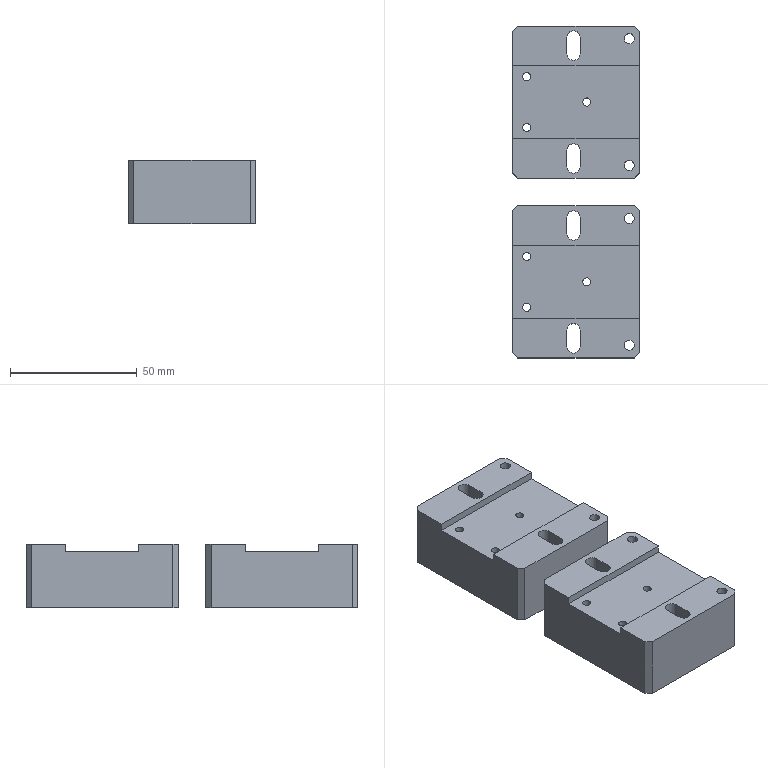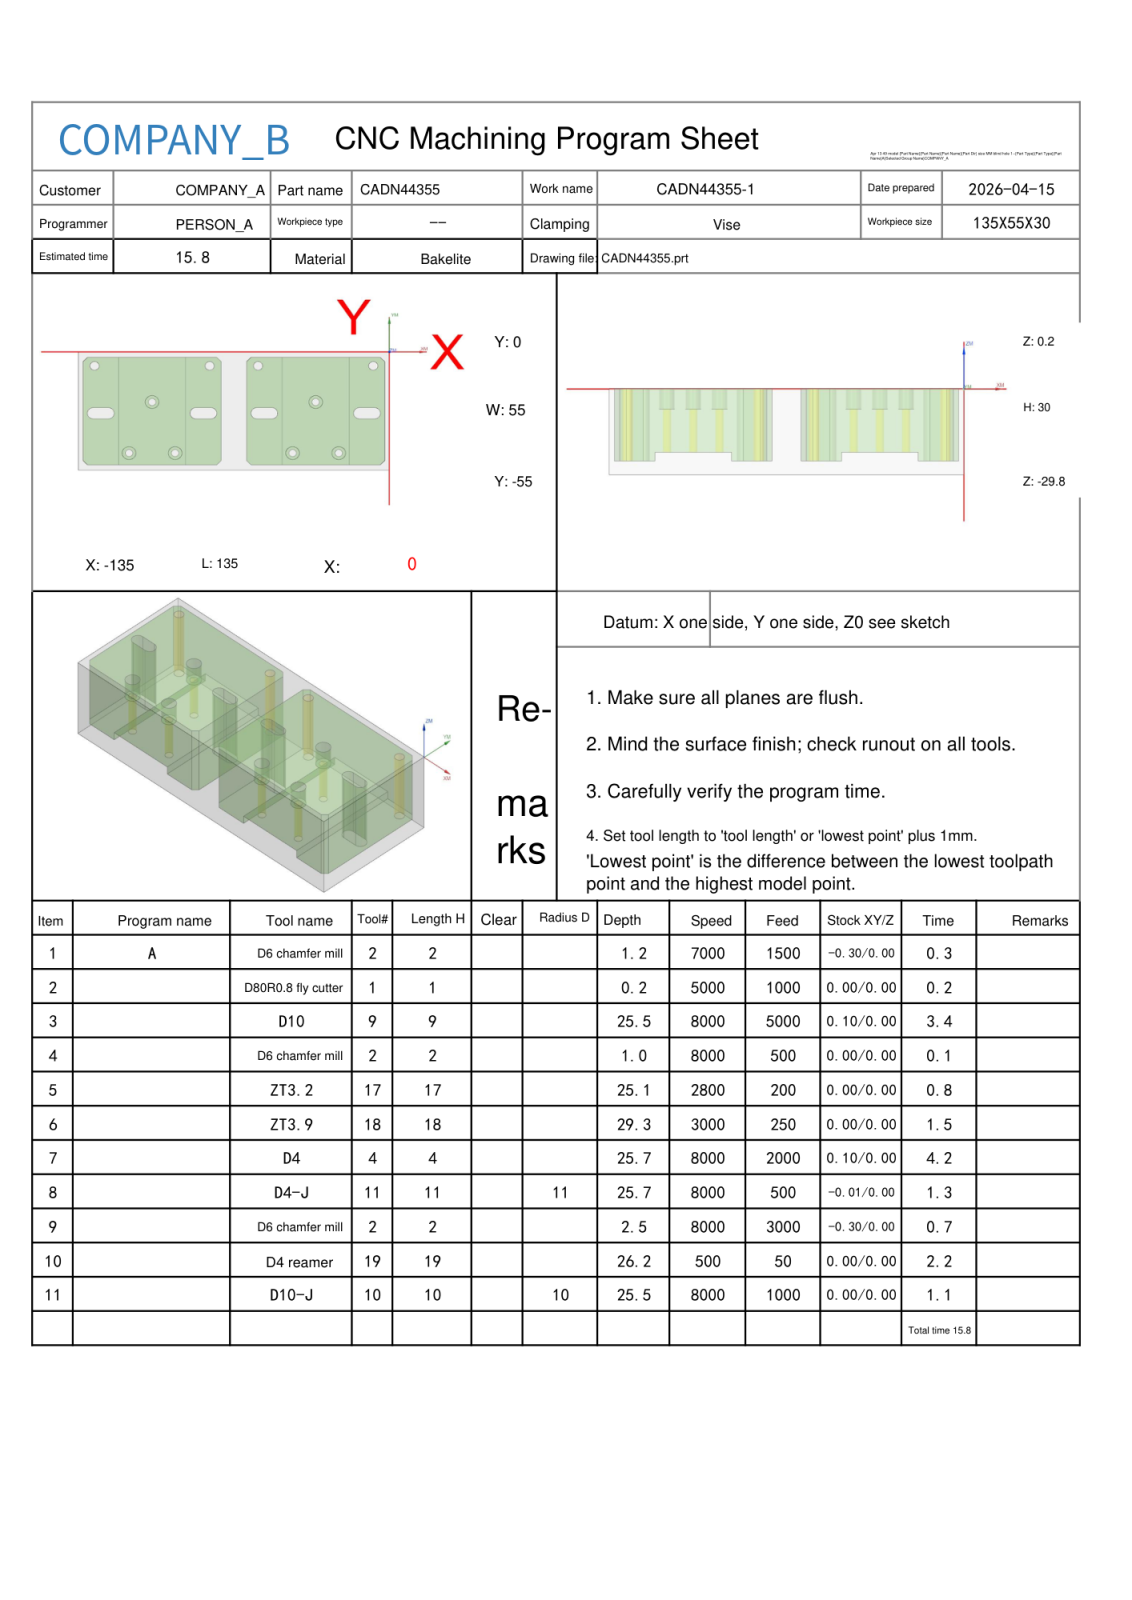NC program | NX | posted by the shop | part box 50 x 131 x 25 mm
Lines 4078 to 5183 of 5183:
N8 T11 M06
(D4-J  D=4. R=0. H=11 ce=0.00 di=0.00)
G00 G90 G54 X-42. Y-47. M03 S8000
G43 H11 Z20.
M08
Z.5
G41 D11
G01 X-41.815 Y-46.923 F500.
G03 X-41.52 Y-46.48 I-.185 J.443
X-42. Y-46. I-.48 J0.0
X-42. Y-46. Z-4.5 I0.0 J-1.
X-42. Y-48. Z-7. I0.0 J-1.
X-41. Y-47. I0.0 J1.
X-42. Y-46. I-1. J0.0
X-43. Y-47. I0.0 J-1.
X-42. Y-48. I1. J0.0
X-41.52 Y-47.52 I0.0 J.48
X-41.815 Y-47.077 I-.48 J0.0
G01 G40 X-42. Y-47.
G00 Z20.
X-22.
Z.5
G41 D11
G01 X-21.815 Y-46.923
G03 X-21.52 Y-46.48 I-.185 J.443
X-22. Y-46. I-.48 J0.0
X-22. Y-46. Z-4.5 I0.0 J-1.
X-22. Y-48. Z-7. I0.0 J-1.
X-21. Y-47. I0.0 J1.
X-22. Y-46. I-1. J0.0
X-23. Y-47. I0.0 J-1.
X-22. Y-48. I1. J0.0
X-21.52 Y-47.52 I0.0 J.48
X-21.815 Y-47.077 I-.48 J0.0
G01 G40 X-22. Y-47.
G00 Z20.
X-32. Y-23.3
Z.5
G41 D11
G01 X-31.815 Y-23.223
G03 X-31.52 Y-22.78 I-.185 J.443
X-32. Y-22.3 I-.48 J0.0
X-32. Y-22.3 Z-4.5 I0.0 J-1.
X-32. Y-24.3 Z-7. I0.0 J-1.
X-31. Y-23.3 I0.0 J1.
X-32. Y-22.3 I-1. J0.0
X-33. Y-23.3 I0.0 J-1.
X-32. Y-24.3 I1. J0.0
X-31.52 Y-23.82 I0.0 J.48
X-31.815 Y-23.377 I-.48 J0.0
G01 G40 X-32. Y-23.3
G00 Z20.
X-93. Y-47.
Z.5
G41 D11
G01 X-92.815 Y-46.923
G03 X-92.52 Y-46.48 I-.185 J.443
X-93. Y-46. I-.48 J0.0
X-93. Y-46. Z-4.5 I0.0 J-1.
X-93. Y-48. Z-7. I0.0 J-1.
X-92. Y-47. I0.0 J1.
X-93. Y-46. I-1. J0.0
X-94. Y-47. I0.0 J-1.
X-93. Y-48. I1. J0.0
X-92.52 Y-47.52 I0.0 J.48
X-92.815 Y-47.077 I-.48 J0.0
G01 G40 X-93. Y-47.
G00 Z20.
X-113.
Z.5
G41 D11
G01 X-112.815 Y-46.923
G03 X-112.52 Y-46.48 I-.185 J.443
X-113. Y-46. I-.48 J0.0
X-113. Y-46. Z-4.5 I0.0 J-1.
X-113. Y-48. Z-7. I0.0 J-1.
X-112. Y-47. I0.0 J1.
X-113. Y-46. I-1. J0.0
X-114. Y-47. I0.0 J-1.
X-113. Y-48. I1. J0.0
X-112.52 Y-47.52 I0.0 J.48
X-112.815 Y-47.077 I-.48 J0.0
G01 G40 X-113. Y-47.
G00 Z20.
X-103. Y-23.3
Z.5
G41 D11
G01 X-102.815 Y-23.223
G03 X-102.52 Y-22.78 I-.185 J.443
X-103. Y-22.3 I-.48 J0.0
X-103. Y-22.3 Z-4.5 I0.0 J-1.
X-103. Y-24.3 Z-7. I0.0 J-1.
X-102. Y-23.3 I0.0 J1.
X-103. Y-22.3 I-1. J0.0
X-104. Y-23.3 I0.0 J-1.
X-103. Y-24.3 I1. J0.0
X-102.52 Y-23.82 I0.0 J.48
X-102.815 Y-23.377 I-.48 J0.0
G01 G40 X-103. Y-23.3
G00 Z20.
G00 G90 X-9.525 Y-28.14 M03 S6000
Z20.
Z-3.75
G01 Z-4.25 F500.
G41 D11
Y-28.09
G03 X-9.725 Y-27.89 I-.2 J0.0
G01 X-12.95
G03 X-13.56 Y-28.5 I0.0 J-.61
X-12.95 Y-29.11 I.61 J0.0
G01 X-6.5
G03 X-5.89 Y-28.5 I0.0 J.61
X-6.5 Y-27.89 I-.61 J0.0
G01 X-9.725
X-10.225
G03 X-10.425 Y-28.09 I0.0 J-.2
G01 G40 Y-28.14
Z-3.75
G00 Z1.
X-9.525
Z-8.
G01 Z-8.5
G41 D11
Y-28.09
G03 X-9.725 Y-27.89 I-.2 J0.0
G01 X-12.95
G03 X-13.56 Y-28.5 I0.0 J-.61
X-12.95 Y-29.11 I.61 J0.0
G01 X-6.5
G03 X-5.89 Y-28.5 I0.0 J.61
X-6.5 Y-27.89 I-.61 J0.0
G01 X-9.725
X-10.225
G03 X-10.425 Y-28.09 I0.0 J-.2
G01 G40 Y-28.14
Z-8.
G00 Z-3.25
X-9.525
Z-12.25
G01 Z-12.75
G41 D11
Y-28.09
G03 X-9.725 Y-27.89 I-.2 J0.0
G01 X-12.95
G03 X-13.56 Y-28.5 I0.0 J-.61
X-12.95 Y-29.11 I.61 J0.0
G01 X-6.5
G03 X-5.89 Y-28.5 I0.0 J.61
X-6.5 Y-27.89 I-.61 J0.0
G01 X-9.725
X-10.225
G03 X-10.425 Y-28.09 I0.0 J-.2
G01 G40 Y-28.14
Z-12.25
G00 Z-7.5
X-9.525
Z-16.5
G01 Z-17.
G41 D11
Y-28.09
G03 X-9.725 Y-27.89 I-.2 J0.0
G01 X-12.95
G03 X-13.56 Y-28.5 I0.0 J-.61
X-12.95 Y-29.11 I.61 J0.0
G01 X-6.5
G03 X-5.89 Y-28.5 I0.0 J.61
X-6.5 Y-27.89 I-.61 J0.0
G01 X-9.725
X-10.225
G03 X-10.425 Y-28.09 I0.0 J-.2
G01 G40 Y-28.14
Z-16.5
G00 Z-11.75
X-9.525
Z-20.75
G01 Z-21.25
G41 D11
Y-28.09
G03 X-9.725 Y-27.89 I-.2 J0.0
G01 X-12.95
G03 X-13.56 Y-28.5 I0.0 J-.61
X-12.95 Y-29.11 I.61 J0.0
G01 X-6.5
G03 X-5.89 Y-28.5 I0.0 J.61
X-6.5 Y-27.89 I-.61 J0.0
G01 X-9.725
X-10.225
G03 X-10.425 Y-28.09 I0.0 J-.2
G01 G40 Y-28.14
Z-20.75
G00 Z-16.
X-9.525
Z-25.
G01 Z-25.5
G41 D11
Y-28.09
G03 X-9.725 Y-27.89 I-.2 J0.0
G01 X-12.95
G03 X-13.56 Y-28.5 I0.0 J-.61
X-12.95 Y-29.11 I.61 J0.0
G01 X-6.5
G03 X-5.89 Y-28.5 I0.0 J.61
X-6.5 Y-27.89 I-.61 J0.0
G01 X-9.725
X-10.225
G03 X-10.425 Y-28.09 I0.0 J-.2
G01 G40 Y-28.14
Z-25.
G00 Z20.
X-54.475 Y-28.86
Z-3.75
G01 Z-4.25
G41 D11
Y-28.91
G03 X-54.275 Y-29.11 I.2 J0.0
G01 X-51.05
G03 X-50.44 Y-28.5 I0.0 J.61
X-51.05 Y-27.89 I-.61 J0.0
G01 X-57.5
G03 X-58.11 Y-28.5 I0.0 J-.61
X-57.5 Y-29.11 I.61 J0.0
G01 X-54.275
X-53.775
G03 X-53.575 Y-28.91 I0.0 J.2
G01 G40 Y-28.86
Z-3.75
G00 Z1.
X-54.475
Z-8.
G01 Z-8.5
G41 D11
Y-28.91
G03 X-54.275 Y-29.11 I.2 J0.0
G01 X-51.05
G03 X-50.44 Y-28.5 I0.0 J.61
X-51.05 Y-27.89 I-.61 J0.0
G01 X-57.5
G03 X-58.11 Y-28.5 I0.0 J-.61
X-57.5 Y-29.11 I.61 J0.0
G01 X-54.275
X-53.775
G03 X-53.575 Y-28.91 I0.0 J.2
G01 G40 Y-28.86
Z-8.
G00 Z-3.25
X-54.475
Z-12.25
G01 Z-12.75
G41 D11
Y-28.91
G03 X-54.275 Y-29.11 I.2 J0.0
G01 X-51.05
G03 X-50.44 Y-28.5 I0.0 J.61
X-51.05 Y-27.89 I-.61 J0.0
G01 X-57.5
G03 X-58.11 Y-28.5 I0.0 J-.61
X-57.5 Y-29.11 I.61 J0.0
G01 X-54.275
X-53.775
G03 X-53.575 Y-28.91 I0.0 J.2
G01 G40 Y-28.86
Z-12.25
G00 Z-7.5
X-54.475
Z-16.5
G01 Z-17.
G41 D11
Y-28.91
G03 X-54.275 Y-29.11 I.2 J0.0
G01 X-51.05
G03 X-50.44 Y-28.5 I0.0 J.61
X-51.05 Y-27.89 I-.61 J0.0
G01 X-57.5
G03 X-58.11 Y-28.5 I0.0 J-.61
X-57.5 Y-29.11 I.61 J0.0
G01 X-54.275
X-53.775
G03 X-53.575 Y-28.91 I0.0 J.2
G01 G40 Y-28.86
Z-16.5
G00 Z-11.75
X-54.475
Z-20.75
G01 Z-21.25
G41 D11
Y-28.91
G03 X-54.275 Y-29.11 I.2 J0.0
G01 X-51.05
G03 X-50.44 Y-28.5 I0.0 J.61
X-51.05 Y-27.89 I-.61 J0.0
G01 X-57.5
G03 X-58.11 Y-28.5 I0.0 J-.61
X-57.5 Y-29.11 I.61 J0.0
G01 X-54.275
X-53.775
G03 X-53.575 Y-28.91 I0.0 J.2
G01 G40 Y-28.86
Z-20.75
G00 Z-16.
X-54.475
Z-25.
G01 Z-25.5
G41 D11
Y-28.91
G03 X-54.275 Y-29.11 I.2 J0.0
G01 X-51.05
G03 X-50.44 Y-28.5 I0.0 J.61
X-51.05 Y-27.89 I-.61 J0.0
G01 X-57.5
G03 X-58.11 Y-28.5 I0.0 J-.61
X-57.5 Y-29.11 I.61 J0.0
G01 X-54.275
X-53.775
G03 X-53.575 Y-28.91 I0.0 J.2
G01 G40 Y-28.86
Z-25.
G00 Z20.
X-80.925
Z-3.75
G01 Z-4.25
G41 D11
Y-28.91
G03 X-80.725 Y-29.11 I.2 J0.0
G01 X-77.5
G03 X-76.89 Y-28.5 I0.0 J.61
X-77.5 Y-27.89 I-.61 J0.0
G01 X-83.95
G03 X-84.56 Y-28.5 I0.0 J-.61
X-83.95 Y-29.11 I.61 J0.0
G01 X-80.725
X-80.225
G03 X-80.025 Y-28.91 I0.0 J.2
G01 G40 Y-28.86
Z-3.75
G00 Z1.
X-80.925
Z-8.
G01 Z-8.5
G41 D11
Y-28.91
G03 X-80.725 Y-29.11 I.2 J0.0
G01 X-77.5
G03 X-76.89 Y-28.5 I0.0 J.61
X-77.5 Y-27.89 I-.61 J0.0
G01 X-83.95
G03 X-84.56 Y-28.5 I0.0 J-.61
X-83.95 Y-29.11 I.61 J0.0
G01 X-80.725
X-80.225
G03 X-80.025 Y-28.91 I0.0 J.2
G01 G40 Y-28.86
Z-8.
G00 Z-3.25
X-80.925
Z-12.25
G01 Z-12.75
G41 D11
Y-28.91
G03 X-80.725 Y-29.11 I.2 J0.0
G01 X-77.5
G03 X-76.89 Y-28.5 I0.0 J.61
X-77.5 Y-27.89 I-.61 J0.0
G01 X-83.95
G03 X-84.56 Y-28.5 I0.0 J-.61
X-83.95 Y-29.11 I.61 J0.0
G01 X-80.725
X-80.225
G03 X-80.025 Y-28.91 I0.0 J.2
G01 G40 Y-28.86
Z-12.25
G00 Z-7.5
X-80.925
Z-16.5
G01 Z-17.
G41 D11
Y-28.91
G03 X-80.725 Y-29.11 I.2 J0.0
G01 X-77.5
G03 X-76.89 Y-28.5 I0.0 J.61
X-77.5 Y-27.89 I-.61 J0.0
G01 X-83.95
G03 X-84.56 Y-28.5 I0.0 J-.61
X-83.95 Y-29.11 I.61 J0.0
G01 X-80.725
X-80.225
G03 X-80.025 Y-28.91 I0.0 J.2
G01 G40 Y-28.86
Z-16.5
G00 Z-11.75
X-80.925
Z-20.75
G01 Z-21.25
G41 D11
Y-28.91
G03 X-80.725 Y-29.11 I.2 J0.0
G01 X-77.5
G03 X-76.89 Y-28.5 I0.0 J.61
X-77.5 Y-27.89 I-.61 J0.0
G01 X-83.95
G03 X-84.56 Y-28.5 I0.0 J-.61
X-83.95 Y-29.11 I.61 J0.0
G01 X-80.725
X-80.225
G03 X-80.025 Y-28.91 I0.0 J.2
G01 G40 Y-28.86
Z-20.75
G00 Z-16.
X-80.925
Z-25.
G01 Z-25.5
G41 D11
Y-28.91
G03 X-80.725 Y-29.11 I.2 J0.0
G01 X-77.5
G03 X-76.89 Y-28.5 I0.0 J.61
X-77.5 Y-27.89 I-.61 J0.0
G01 X-83.95
G03 X-84.56 Y-28.5 I0.0 J-.61
X-83.95 Y-29.11 I.61 J0.0
G01 X-80.725
X-80.225
G03 X-80.025 Y-28.91 I0.0 J.2
G01 G40 Y-28.86
Z-25.
G00 Z20.
X-125.075 Y-28.14
Z-3.75
G01 Z-4.25
G41 D11
Y-28.09
G03 X-125.275 Y-27.89 I-.2 J0.0
G01 X-128.5
G03 X-129.11 Y-28.5 I0.0 J-.61
X-128.5 Y-29.11 I.61 J0.0
G01 X-122.05
G03 X-121.44 Y-28.5 I0.0 J.61
X-122.05 Y-27.89 I-.61 J0.0
G01 X-125.275
X-125.775
G03 X-125.975 Y-28.09 I0.0 J-.2
G01 G40 Y-28.14
Z-3.75
G00 Z1.
X-125.075
Z-8.
G01 Z-8.5
G41 D11
Y-28.09
G03 X-125.275 Y-27.89 I-.2 J0.0
G01 X-128.5
G03 X-129.11 Y-28.5 I0.0 J-.61
X-128.5 Y-29.11 I.61 J0.0
G01 X-122.05
G03 X-121.44 Y-28.5 I0.0 J.61
X-122.05 Y-27.89 I-.61 J0.0
G01 X-125.275
X-125.775
G03 X-125.975 Y-28.09 I0.0 J-.2
G01 G40 Y-28.14
Z-8.
G00 Z-3.25
X-125.075
Z-12.25
G01 Z-12.75
G41 D11
Y-28.09
G03 X-125.275 Y-27.89 I-.2 J0.0
G01 X-128.5
G03 X-129.11 Y-28.5 I0.0 J-.61
X-128.5 Y-29.11 I.61 J0.0
G01 X-122.05
G03 X-121.44 Y-28.5 I0.0 J.61
X-122.05 Y-27.89 I-.61 J0.0
G01 X-125.275
X-125.775
G03 X-125.975 Y-28.09 I0.0 J-.2
G01 G40 Y-28.14
Z-12.25
G00 Z-7.5
X-125.075
Z-16.5
G01 Z-17.
G41 D11
Y-28.09
G03 X-125.275 Y-27.89 I-.2 J0.0
G01 X-128.5
G03 X-129.11 Y-28.5 I0.0 J-.61
X-128.5 Y-29.11 I.61 J0.0
G01 X-122.05
G03 X-121.44 Y-28.5 I0.0 J.61
X-122.05 Y-27.89 I-.61 J0.0
G01 X-125.275
X-125.775
G03 X-125.975 Y-28.09 I0.0 J-.2
G01 G40 Y-28.14
Z-16.5
G00 Z-11.75
X-125.075
Z-20.75
G01 Z-21.25
G41 D11
Y-28.09
G03 X-125.275 Y-27.89 I-.2 J0.0
G01 X-128.5
G03 X-129.11 Y-28.5 I0.0 J-.61
X-128.5 Y-29.11 I.61 J0.0
G01 X-122.05
G03 X-121.44 Y-28.5 I0.0 J.61
X-122.05 Y-27.89 I-.61 J0.0
G01 X-125.275
X-125.775
G03 X-125.975 Y-28.09 I0.0 J-.2
G01 G40 Y-28.14
Z-20.75
G00 Z-16.
X-125.075
Z-25.
G01 Z-25.5
G41 D11
Y-28.09
G03 X-125.275 Y-27.89 I-.2 J0.0
G01 X-128.5
G03 X-129.11 Y-28.5 I0.0 J-.61
X-128.5 Y-29.11 I.61 J0.0
G01 X-122.05
G03 X-121.44 Y-28.5 I0.0 J.61
X-122.05 Y-27.89 I-.61 J0.0
G01 X-125.275
X-125.775
G03 X-125.975 Y-28.09 I0.0 J-.2
G01 G40 Y-28.14
Z-25.
G00 Z20.
G91 G28 Z0.0
M05
M09
G91 G28 Z0.0
M01
N9 T02 M06
(D6 chamfer mill  D=6. R=0. H=02 ce=0.00 di=0.00)
G00 G90 G54 X-31.75 Y-54.628 M03 S8000
G43 H02 Z20.
M08
Z2.099
G01 Z-1.5 F3000.
G03 X-31.67 Y-54.328 I-.52 J.3
X-31.97 Y-53.808 I-.6 J0.0
G01 X-32. Y-53.8
X-60.
X-60.254 Y-53.775
X-60.497 Y-53.701
X-60.722 Y-53.581
X-60.919 Y-53.419
X-62.919 Y-51.419
X-63.081 Y-51.222
X-63.201 Y-50.997
X-63.275 Y-50.754
X-63.3 Y-50.5
Y-4.5
X-63.275 Y-4.246
X-63.201 Y-4.003
X-63.081 Y-3.778
X-62.919 Y-3.581
X-60.919 Y-1.581
X-60.722 Y-1.419
X-60.497 Y-1.299
X-60.254 Y-1.225
X-60. Y-1.2
X-4.
X-3.746 Y-1.225
X-3.503 Y-1.299
X-3.278 Y-1.419
X-3.081 Y-1.581
X-1.081 Y-3.581
X-.919 Y-3.778
X-.799 Y-4.003
X-.725 Y-4.246
X-.7 Y-4.5
Y-50.5
X-.725 Y-50.754
X-.799 Y-50.997
X-.919 Y-51.222
X-1.081 Y-51.419
X-3.081 Y-53.419
X-3.278 Y-53.581
X-3.503 Y-53.701
X-3.746 Y-53.775
X-4. Y-53.8
X-32.
X-32.03 Y-53.808
G03 X-32.33 Y-54.328 I.3 J-.52
X-32.25 Y-54.628 I.6 J0.0
G01 Z2.099
G00 Z20.
X-9.475 Y-28.028
Z2.099
G01 Z-1.5
G03 X-9.395 Y-27.728 I-.52 J.3
X-9.695 Y-27.208 I-.6 J0.0
G01 X-9.725 Y-27.2
X-12.95
G03 X-14.25 Y-28.5 I0.0 J-1.3
X-12.95 Y-29.8 I1.3 J0.0
G01 X-6.5
G03 X-5.2 Y-28.5 I0.0 J1.3
X-6.5 Y-27.2 I-1.3 J0.0
G01 X-9.725
X-9.755 Y-27.208
G03 X-10.055 Y-27.728 I.3 J-.52
X-9.975 Y-28.028 I.6 J0.0
G01 Z2.099
G00 Z20.
X-54.025
Z2.099
G01 Z-1.5
G03 X-53.945 Y-27.728 I-.52 J.3
X-54.245 Y-27.208 I-.6 J0.0
G01 X-54.275 Y-27.2
X-57.5
G03 X-58.8 Y-28.5 I0.0 J-1.3
X-57.5 Y-29.8 I1.3 J0.0
G01 X-51.05
G03 X-49.75 Y-28.5 I0.0 J1.3
X-51.05 Y-27.2 I-1.3 J0.0
G01 X-54.275
X-54.305 Y-27.208
G03 X-54.605 Y-27.728 I.3 J-.52
X-54.525 Y-28.028 I.6 J0.0
G01 Z2.099
G00 Z20.
X-102.75 Y-54.628
Z2.099
G01 Z-1.5
G03 X-102.67 Y-54.328 I-.52 J.3
X-102.97 Y-53.808 I-.6 J0.0
G01 X-103. Y-53.8
X-131.
X-131.254 Y-53.775
X-131.497 Y-53.701
X-131.722 Y-53.581
X-131.919 Y-53.419
X-133.919 Y-51.419
X-134.081 Y-51.222
X-134.201 Y-50.997
X-134.275 Y-50.754
X-134.3 Y-50.5
Y-4.5
X-134.275 Y-4.246
X-134.201 Y-4.003
X-134.081 Y-3.778
X-133.919 Y-3.581
X-131.919 Y-1.581
X-131.722 Y-1.419
X-131.497 Y-1.299
X-131.254 Y-1.225
X-131. Y-1.2
X-75.
X-74.746 Y-1.225
X-74.503 Y-1.299
X-74.278 Y-1.419
X-74.081 Y-1.581
X-72.081 Y-3.581
X-71.919 Y-3.778
X-71.799 Y-4.003
X-71.725 Y-4.246
X-71.7 Y-4.5
Y-50.5
X-71.725 Y-50.754
X-71.799 Y-50.997
X-71.919 Y-51.222
X-72.081 Y-51.419
X-74.081 Y-53.419
X-74.278 Y-53.581
X-74.503 Y-53.701
X-74.746 Y-53.775
X-75. Y-53.8
X-103.
X-103.03 Y-53.808
G03 X-103.33 Y-54.328 I.3 J-.52
X-103.25 Y-54.628 I.6 J0.0
G01 Z2.099
G00 Z20.
X-80.475 Y-28.028
Z2.099
G01 Z-1.5
G03 X-80.395 Y-27.728 I-.52 J.3
X-80.695 Y-27.208 I-.6 J0.0
G01 X-80.725 Y-27.2
X-83.95
G03 X-85.25 Y-28.5 I0.0 J-1.3
X-83.95 Y-29.8 I1.3 J0.0
G01 X-77.5
G03 X-76.2 Y-28.5 I0.0 J1.3
X-77.5 Y-27.2 I-1.3 J0.0
G01 X-80.725
X-80.755 Y-27.208
G03 X-81.055 Y-27.728 I.3 J-.52
X-80.975 Y-28.028 I.6 J0.0
G01 Z2.099
G00 Z20.
X-125.025
Z2.099
G01 Z-1.5
G03 X-124.945 Y-27.728 I-.52 J.3
X-125.245 Y-27.208 I-.6 J0.0
G01 X-125.275 Y-27.2
X-128.5
G03 X-129.8 Y-28.5 I0.0 J-1.3
X-128.5 Y-29.8 I1.3 J0.0
G01 X-122.05
G03 X-120.75 Y-28.5 I0.0 J1.3
X-122.05 Y-27.2 I-1.3 J0.0
G01 X-125.275
X-125.305 Y-27.208
G03 X-125.605 Y-27.728 I.3 J-.52
X-125.525 Y-28.028 I.6 J0.0
G01 Z2.099
G00 Z20.
G00 G90 X-7. Y-6.5 M03 S8000
Z20.
G98 G81 X-7. Y-6.5 Z-2.3 R3. F500.
X-57.
X-78.
X-128.
G80
G00 Z20.
G00 G90 X-101.019 Y-22.13 M03 S8000
Z20.
Z2.5
G01 X-101.067 Y-22.048 Z2.465 F500.
X-101.264 Y-21.787 Z2.346
X-101.496 Y-21.556 Z2.227
X-101.759 Y-21.36 Z2.108
X-102.046 Y-21.204 Z1.989
X-102.353 Y-21.09 Z1.87
X-102.673 Y-21.02 Z1.75
X-103. Y-20.997 Z1.631
X-103.327 Y-21.02 Z1.512
X-103.647 Y-21.09 Z1.393
X-103.954 Y-21.204 Z1.274
X-104.241 Y-21.36 Z1.154
X-104.504 Y-21.556 Z1.035
X-104.736 Y-21.787 Z.916
X-104.933 Y-22.048 Z.797
X-105.051 Y-22.252 Z.711
X-105.179 Y-22.553 Z.592
X-105.262 Y-22.87 Z.473
X-105.301 Y-23.195 Z.354
X-105.292 Y-23.522 Z.235
X-105.238 Y-23.845 Z.115
X-105.138 Y-24.157 Z-.004
X-104.994 Y-24.452 Z-.123
X-104.811 Y-24.723 Z-.242
X-104.591 Y-24.965 Z-.361
X-104.339 Y-25.174 Z-.48
X-104.059 Y-25.345 Z-.6
X-103.759 Y-25.474 Z-.719
X-103.443 Y-25.56 Z-.838
X-103.118 Y-25.6 Z-.957
X-103. Z-1.
G03 X-100.7 Y-23.3 I0.0 J2.3
X-103. Y-21. I-2.3 J0.0
X-105.3 Y-23.3 I0.0 J-2.3
X-103. Y-25.6 I2.3 J0.0
X-102.504 Y-25.546 I0.0 J2.3
G01 Z1.5
G00 Z20.
X-111.019 Y-45.83
Z2.5
G01 X-111.067 Y-45.748 Z2.465
X-111.264 Y-45.487 Z2.346
X-111.496 Y-45.256 Z2.227
X-111.759 Y-45.06 Z2.108
X-112.046 Y-44.904 Z1.989
X-112.353 Y-44.79 Z1.87
X-112.673 Y-44.72 Z1.75
X-113. Y-44.697 Z1.631
X-113.327 Y-44.72 Z1.512
X-113.647 Y-44.79 Z1.393
X-113.954 Y-44.904 Z1.274
X-114.241 Y-45.06 Z1.154
X-114.504 Y-45.256 Z1.035
X-114.736 Y-45.487 Z.916
X-114.933 Y-45.748 Z.797
X-115.051 Y-45.952 Z.711
X-115.179 Y-46.253 Z.592
X-115.262 Y-46.57 Z.473
X-115.301 Y-46.895 Z.354
X-115.292 Y-47.222 Z.235
X-115.238 Y-47.545 Z.115
X-115.138 Y-47.857 Z-.004
X-114.994 Y-48.152 Z-.123
X-114.811 Y-48.423 Z-.242
X-114.591 Y-48.665 Z-.361
X-114.339 Y-48.874 Z-.48
X-114.059 Y-49.045 Z-.6
X-113.759 Y-49.174 Z-.719
X-113.443 Y-49.26 Z-.838
X-113.118 Y-49.3 Z-.957
X-113. Z-1.
G03 X-110.7 Y-47. I0.0 J2.3
X-113. Y-44.7 I-2.3 J0.0
X-115.3 Y-47. I0.0 J-2.3
X-113. Y-49.3 I2.3 J0.0
X-112.504 Y-49.246 I0.0 J2.3
G01 Z1.5
G00 Z20.
X-91.019 Y-45.83
Z2.5
G01 X-91.067 Y-45.748 Z2.465
X-91.264 Y-45.487 Z2.346
X-91.496 Y-45.256 Z2.227
X-91.759 Y-45.06 Z2.108
X-92.046 Y-44.904 Z1.989
X-92.353 Y-44.79 Z1.87
X-92.673 Y-44.72 Z1.75
X-93. Y-44.697 Z1.631
X-93.327 Y-44.72 Z1.512
X-93.647 Y-44.79 Z1.393
X-93.954 Y-44.904 Z1.274
X-94.241 Y-45.06 Z1.154
X-94.504 Y-45.256 Z1.035
X-94.736 Y-45.487 Z.916
X-94.933 Y-45.748 Z.797
X-95.051 Y-45.952 Z.711
X-95.179 Y-46.253 Z.592
X-95.262 Y-46.57 Z.473
X-95.301 Y-46.895 Z.354
X-95.292 Y-47.222 Z.235
X-95.238 Y-47.545 Z.115
X-95.138 Y-47.857 Z-.004
X-94.994 Y-48.152 Z-.123
X-94.811 Y-48.423 Z-.242
X-94.591 Y-48.665 Z-.361
X-94.339 Y-48.874 Z-.48
X-94.059 Y-49.045 Z-.6
X-93.759 Y-49.174 Z-.719
X-93.443 Y-49.26 Z-.838
X-93.118 Y-49.3 Z-.957
X-93. Z-1.
G03 X-90.7 Y-47. I0.0 J2.3
X-93. Y-44.7 I-2.3 J0.0
X-95.3 Y-47. I0.0 J-2.3
X-93. Y-49.3 I2.3 J0.0
X-92.504 Y-49.246 I0.0 J2.3
G01 Z1.5
G00 Z20.
X-40.019 Y-45.83
Z2.5
G01 X-40.067 Y-45.748 Z2.465
X-40.264 Y-45.487 Z2.346
X-40.496 Y-45.256 Z2.227
X-40.759 Y-45.06 Z2.108
X-41.046 Y-44.904 Z1.989
X-41.353 Y-44.79 Z1.87
X-41.673 Y-44.72 Z1.75
X-42. Y-44.697 Z1.631
X-42.327 Y-44.72 Z1.512
X-42.647 Y-44.79 Z1.393
X-42.954 Y-44.904 Z1.274
X-43.241 Y-45.06 Z1.154
X-43.504 Y-45.256 Z1.035
X-43.736 Y-45.487 Z.916
X-43.933 Y-45.748 Z.797
X-44.051 Y-45.952 Z.711
X-44.179 Y-46.253 Z.592
X-44.262 Y-46.57 Z.473
X-44.301 Y-46.895 Z.354
X-44.292 Y-47.222 Z.235
X-44.238 Y-47.545 Z.115
X-44.138 Y-47.857 Z-.004
X-43.994 Y-48.152 Z-.123
X-43.811 Y-48.423 Z-.242
X-43.591 Y-48.665 Z-.361
X-43.339 Y-48.874 Z-.48
X-43.059 Y-49.045 Z-.6
X-42.759 Y-49.174 Z-.719
X-42.443 Y-49.26 Z-.838
X-42.118 Y-49.3 Z-.957
X-42. Z-1.
G03 X-39.7 Y-47. I0.0 J2.3
X-42. Y-44.7 I-2.3 J0.0
X-44.3 Y-47. I0.0 J-2.3
X-42. Y-49.3 I2.3 J0.0
X-41.504 Y-49.246 I0.0 J2.3
G01 Z1.5
G00 Z20.
X-20.019 Y-45.83
Z2.5
G01 X-20.067 Y-45.748 Z2.465
X-20.264 Y-45.487 Z2.346
X-20.496 Y-45.256 Z2.227
X-20.759 Y-45.06 Z2.108
X-21.046 Y-44.904 Z1.989
X-21.353 Y-44.79 Z1.87
X-21.673 Y-44.72 Z1.75
X-22. Y-44.697 Z1.631
X-22.327 Y-44.72 Z1.512
X-22.647 Y-44.79 Z1.393
X-22.954 Y-44.904 Z1.274
X-23.241 Y-45.06 Z1.154
X-23.504 Y-45.256 Z1.035
X-23.736 Y-45.487 Z.916
X-23.933 Y-45.748 Z.797
X-24.051 Y-45.952 Z.711
X-24.179 Y-46.253 Z.592
X-24.262 Y-46.57 Z.473
X-24.301 Y-46.895 Z.354
X-24.292 Y-47.222 Z.235
X-24.238 Y-47.545 Z.115
X-24.138 Y-47.857 Z-.004
X-23.994 Y-48.152 Z-.123
X-23.811 Y-48.423 Z-.242
X-23.591 Y-48.665 Z-.361
X-23.339 Y-48.874 Z-.48
X-23.059 Y-49.045 Z-.6
X-22.759 Y-49.174 Z-.719
X-22.443 Y-49.26 Z-.838
X-22.118 Y-49.3 Z-.957
X-22. Z-1.
G03 X-19.7 Y-47. I0.0 J2.3
X-22. Y-44.7 I-2.3 J0.0
X-24.3 Y-47. I0.0 J-2.3
X-22. Y-49.3 I2.3 J0.0
X-21.504 Y-49.246 I0.0 J2.3
G01 Z1.5
G00 Z20.
X-30.019 Y-22.13
Z2.5
G01 X-30.067 Y-22.048 Z2.465
X-30.264 Y-21.787 Z2.346
X-30.496 Y-21.556 Z2.227
X-30.759 Y-21.36 Z2.108
X-31.046 Y-21.204 Z1.989
X-31.353 Y-21.09 Z1.87
X-31.673 Y-21.02 Z1.75
X-32. Y-20.997 Z1.631
X-32.327 Y-21.02 Z1.512
X-32.647 Y-21.09 Z1.393
X-32.954 Y-21.204 Z1.274
X-33.241 Y-21.36 Z1.154
X-33.504 Y-21.556 Z1.035
X-33.736 Y-21.787 Z.916
X-33.933 Y-22.048 Z.797
X-34.051 Y-22.252 Z.711
X-34.179 Y-22.553 Z.592
X-34.262 Y-22.87 Z.473
X-34.301 Y-23.195 Z.354
X-34.292 Y-23.522 Z.235
X-34.238 Y-23.845 Z.115
X-34.138 Y-24.157 Z-.004
X-33.994 Y-24.452 Z-.123
X-33.811 Y-24.723 Z-.242
X-33.591 Y-24.965 Z-.361
X-33.339 Y-25.174 Z-.48
X-33.059 Y-25.345 Z-.6
X-32.759 Y-25.474 Z-.719
X-32.443 Y-25.56 Z-.838
X-32.118 Y-25.6 Z-.957
X-32. Z-1.
G03 X-29.7 Y-23.3 I0.0 J2.3
X-32. Y-21. I-2.3 J0.0
X-34.3 Y-23.3 I0.0 J-2.3
X-32. Y-25.6 I2.3 J0.0
X-31.504 Y-25.546 I0.0 J2.3
G01 Z1.5
G00 Z20.
G91 G28 Z0.0
M05
M09
G91 G28 Z0.0
M01
N10 T19 M06
(D4 reamer D=4. DR_a=180 H=19)
G00 G90 G54 X-7. Y-6.5 M03 S500
G43 H19 Z20.
M08
G98 G81 X-7. Y-6.5 Z-26. R1. F50.
X-57.
X-78.
X-128.
G80
G00 Z20.
G91 G28 Z0.0
M05
M09
G91 G28 Z0.0
M01
N11 T10 M06
(D10-J  D=10. R=0. H=10 ce=0.00 di=0.00)
G00 G90 G54 X-61.013 Y3.616 M03 S8000
G43 H10 Z20.
M08
Z-12.15
G01 Z-12.65 F1000.
G41 D10
X-60.997 Y3.417
G03 X-60. Y2.5 I.997 J.083
G01 X-4.
G02 X-.464 Y1.036 I0.0 J-5.
G01 X1.536 Y-.964
G02 X3. Y-4.5 I-3.536 J-3.536
G01 Y-50.5
G02 X1.536 Y-54.036 I-5. J0.0
G01 X-.464 Y-56.036
G02 X-4. Y-57.5 I-3.536 J3.536
G01 X-60.
G02 X-63.536 Y-56.036 I0.0 J5.
G01 X-65.536 Y-54.036
G02 X-67. Y-50.5 I3.536 J3.536
G01 Y-4.5
G02 X-65.536 Y-.964 I5. J0.0
G01 X-63.536 Y1.036
G02 X-60. Y2.5 I3.536 J-3.536
G01 X-59.5
G03 X-58.5 Y3.5 I0.0 J1.
G01 G40 Y3.7
X-68.095 Y-.708
G41 D10
X-68.263 Y-.818
G03 X-68.717 Y-1.655 I.546 J-.838
X-68.598 Y-2.13 I1. J0.0
G02 X-68. Y-4.499 I-4.402 J-2.37
G01 Y-50.501
G02 X-69.464 Y-54.036 I-5. J.001
G01 X-71.464 Y-56.036
G02 X-75. Y-57.5 I-3.536 J3.536
G01 X-131.
G02 X-134.536 Y-56.036 I0.0 J5.
G01 X-136.536 Y-54.036
G02 X-138. Y-50.5 I3.536 J3.536
G01 Y-4.5
G02 X-136.536 Y-.964 I5. J0.0
G01 X-134.536 Y1.036
G02 X-131. Y2.5 I3.536 J-3.536
G01 X-75.
G02 X-71.464 Y1.036 I0.0 J-5.
G01 X-69.464 Y-.964
G02 X-68.598 Y-2.13 I-3.536 J-3.536
X-68.383 Y-2.581 I-4.402 J-2.37
G03 X-67.46 Y-3.197 I.923 J.384
X-67.076 Y-3.12 I0.0 J1.
G01 G40 X-67.5 Y-2.102
Z-12.15
G00 Z20.
X-132.013 Y3.616
Z-24.8
G01 Z-25.3
G41 D10
X-131.997 Y3.417
G03 X-131. Y2.5 I.997 J.083
G01 X-75.
G02 X-71.464 Y1.036 I0.0 J-5.
G01 X-69.464 Y-.964
G02 X-68. Y-4.499 I-3.536 J-3.536
G01 Y-50.501
G02 X-69.464 Y-54.036 I-5. J.001
G01 X-71.464 Y-56.036
G02 X-75. Y-57.5 I-3.536 J3.536
G01 X-131.
G02 X-134.536 Y-56.036 I0.0 J5.
G01 X-136.536 Y-54.036
G02 X-138. Y-50.5 I3.536 J3.536
G01 Y-4.5
G02 X-136.536 Y-.964 I5. J0.0
G01 X-134.536 Y1.036
G02 X-131. Y2.5 I3.536 J-3.536
G01 X-130.5
G03 X-129.5 Y3.5 I0.0 J1.
G01 G40 Y3.7
Z-24.8
G00 Z20.
X-33.
Z-24.8
G01 Z-25.3
G41 D10
Y3.5
G03 X-32. Y2.5 I1. J0.0
G01 X-4.
G02 X-.464 Y1.036 I0.0 J-5.
G01 X1.536 Y-.964
G02 X3. Y-4.5 I-3.536 J-3.536
G01 Y-50.5
G02 X1.536 Y-54.036 I-5. J0.0
G01 X-.464 Y-56.036
G02 X-4. Y-57.5 I-3.536 J3.536
G01 X-60.
G02 X-63.536 Y-56.036 I0.0 J5.
G01 X-65.536 Y-54.036
G02 X-67. Y-50.5 I3.536 J3.536
G01 Y-4.5
G02 X-65.536 Y-.964 I5. J0.0
G01 X-63.536 Y1.036
G02 X-60. Y2.5 I3.536 J-3.536
G01 X-32.
X-31.5
G03 X-30.5 Y3.5 I0.0 J1.
G01 G40 Y3.7
Z-24.8
G00 Z20.
M05
M09
G91 G28 Z0.0
G91 G28 Y0.0
M30
%